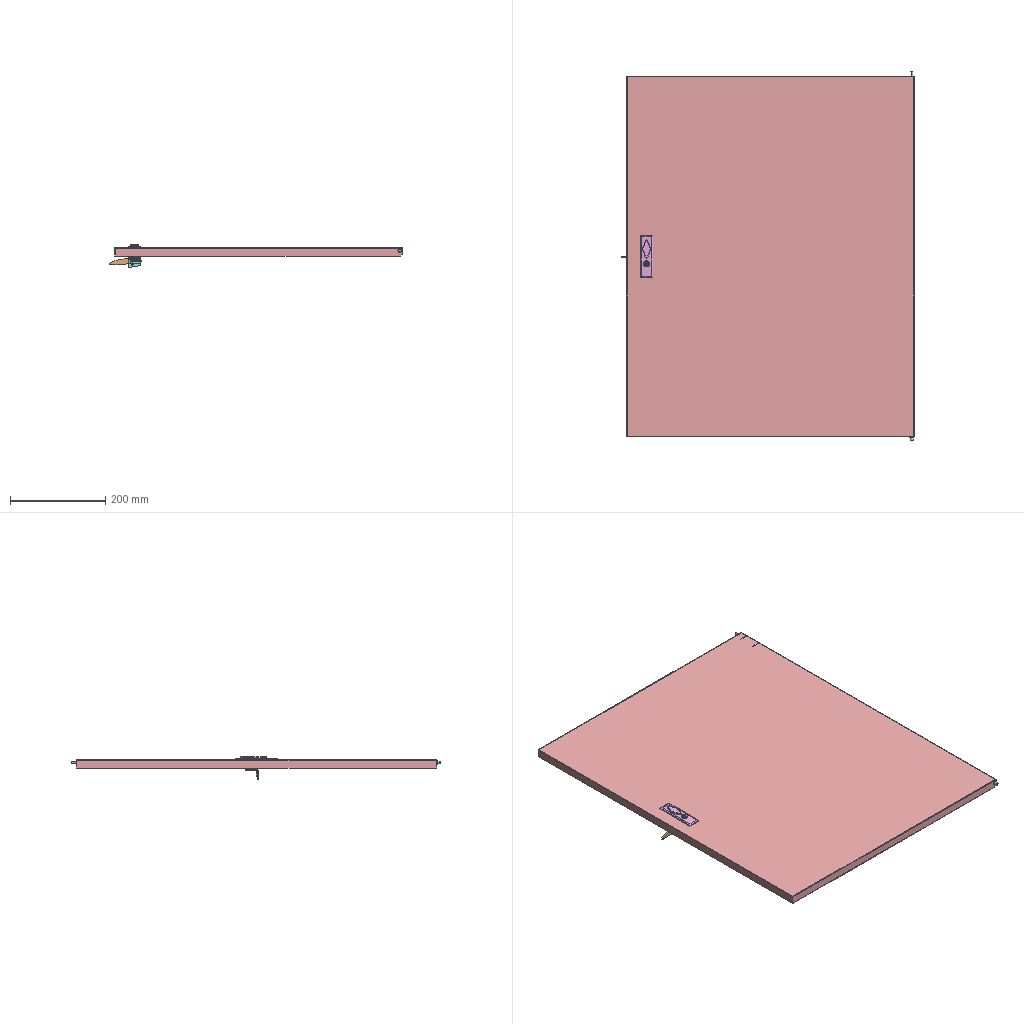Assembly | SolidWorks | 9 different items | 9 placed | box 616 x 776 x 48 mm
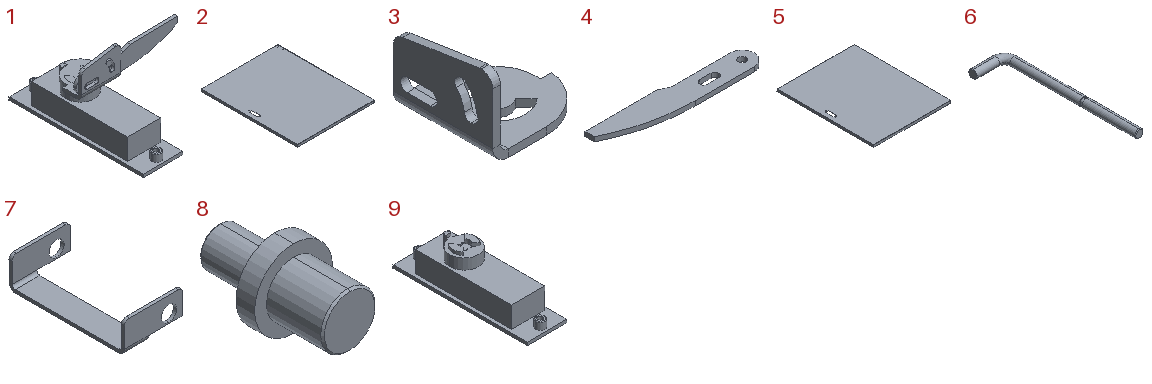Parts list (item | name | quantity | parent item | size | volume | features):
1 | (subassembly) | x1 | - | 67.187 x 89 x 47.503 mm | 33302 mm3 | -
2 | (subassembly) | x1 | - | 605 x 766 x 18 mm | 499858 mm3 | -
3 | - | x1 | in 1 | 26.913 x 26 x 20.503 mm | 1687 mm3 | features ICE 4, EdgeFlange 1, Fillet 1, FlatPattern 1, SMBaseFlange 1, SheetMetal 1
4 | - | x1 | in 1 | 67.25 x 12.5 x 2 mm | 1251 mm3 | features SMBaseFlange 2, FlatPattern 1, ICE 1, SheetMetal 1
5 | - | x1 | - | 605 x 758 x 18 mm | 498938 mm3 | features ICE 4, CornerFeat 1, EdgeFlange 1, FlatPattern 1, SMBaseFlange 1, SheetMetal 1
6 | - | x1 | - | 19.75 x 75.75 x 4.5 mm | 1403 mm3 | features Chamfer 1, RevCut 1, Sweep 1
7 | - | x1 | - | 19 x 37.5 x 10 mm | 570.053 mm3 | features EdgeFlange 2, ICE 2, CornerTrim 1, FlatPattern 1, SMBaseFlange 1, SheetMetal 1
8 | - | x1 | - | 8.3 x 14 x 8.3 mm | 349.252 mm3 | features Chamfer 1, Revolution 1
9 | - | x1 | in 1 | 26.5 x 89 x 29 mm | 30365 mm3 | features ICE 11, Fillet 3, Chamfer 1, Extrusion 1, HoleWzd 1
Mates (type | each side: item.copy, entity, surface, feature):
In the top assembly
Concentric | 5.1 face cylinder Cut-Extrude2 | 8.1 face cylinder Revolve1
Coincident | 5.1 face plane Edge-Flange1 | 8.1 face plane Revolve1
Coincident | 5.1 face plane Base-Flange1 | 7.1 face plane Edge-Flange2
Coincident | 5.1 face plane Edge-Flange1 | 7.1 face plane Edge-Flange2
DistanceDim | 5.1 face plane Edge-Flange1 | 7.1 face plane Edge-Flange2
Coincident | 5.1 face plane Base-Flange1 | 9.1 face plane Boss-Extrude1
Coincident | 5.1 face plane Cut-Extrude1 | 9.1 face plane Boss-Extrude2 | 2 times
Concentric | 5.1 edge | 6.1 face cylinder Sweep1
DistanceDim | 5.1 face plane Edge-Flange1 | 6.1 face plane Sweep1
Parallel | 5.1 face plane Edge-Flange1 | 6.1 plane
In subassembly 1
Coincident | 9.2 face plane Boss-Extrude4 | 3.1 face plane Base-Flange1
Concentric | 9.2 face cylinder Boss-Extrude4 | 3.1 face cylinder Base-Flange1
Coincident | 3.1 face plane Edge-Flange1 | 4.1 face plane Base-Flange1
Coincident | 9.2 face plane Cut-Extrude6 | 3.1 face plane Cut-Extrude2
Concentric | 3.1 face cylinder Cut-Extrude3 | 4.1 face cylinder Base-Flange1